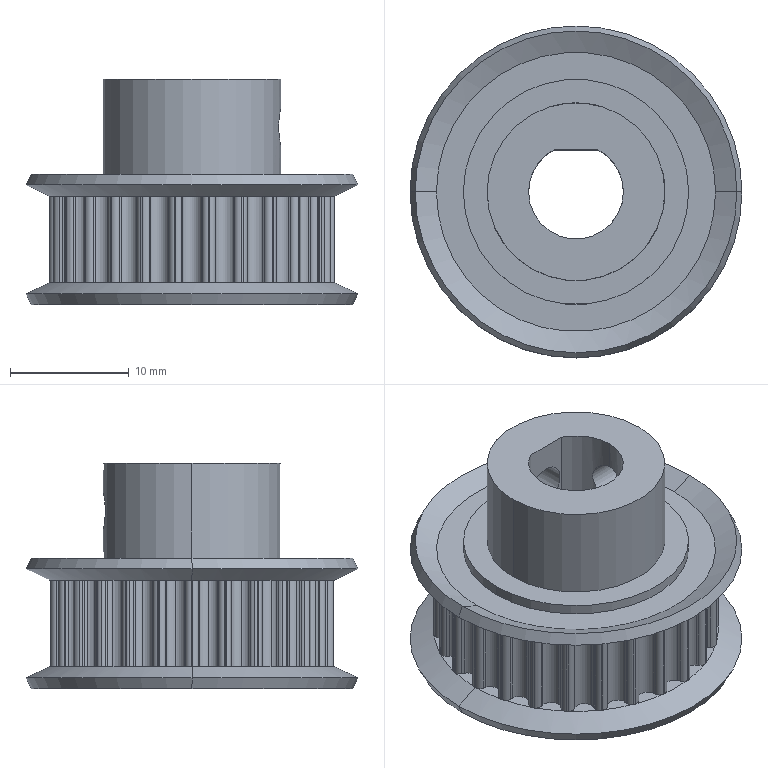Part | NX | features BREP 1 | 1 solid | 312 faces | box 28 x 28 x 19 mm | volume 5118 mm3 | cylinder 190 | plane 110 | cone 12 | commonest cylinder face diameters 1.02 x62 3.04 x52 1.7 x36 24.07 x27 3.3 x4 19 x4